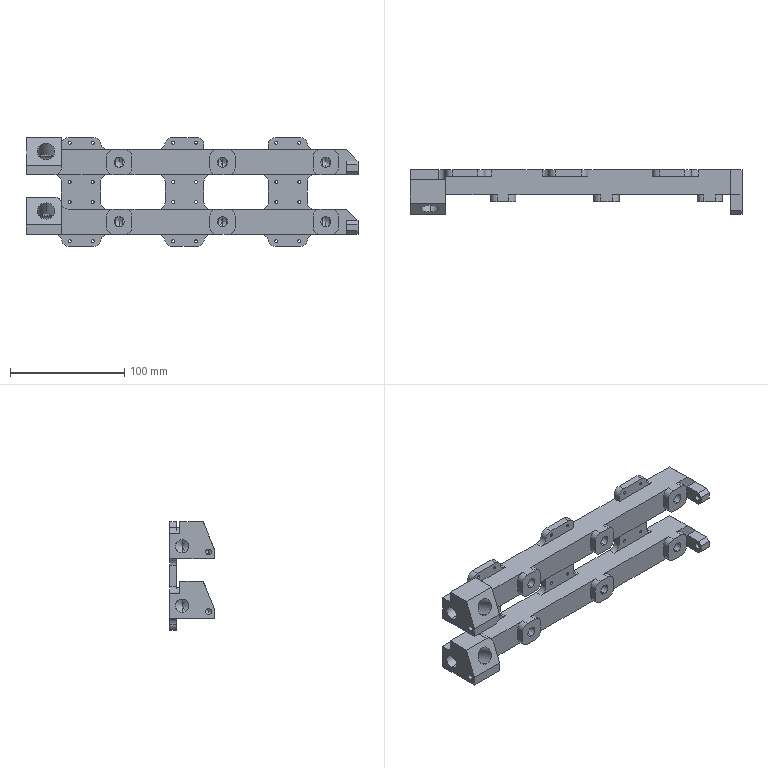CAM job | NX | 3+2 milling, drilling | part box 290 x 39.082 x 95 mm | stock box 300 x 49.082 x 95.918 mm
Tools:
number,name,description,diameter,corner_radius,flute_length,length,flutes
3,V4,定心钻D4,4.0,0.0,43.0,75.0,2
1,V10,定心钻D10,10.0,0.0,87.0,133.0,2
4,D4_J,D4,4.0,0.0,12.0,50.0,2
9,D6,D6,6.0,0.0,16.0,60.0,2
7,D8,D8,8.0,0.0,20.0,60.0,2
4,D8_J,D8,8.0,0.0,20.0,60.0,2
3,D10_J,D10,10.0,0.0,25.0,75.0,2
2,D12,D12,12.0,0.0,30.0,75.0,2
2,D16,D16,16.0,0.0,45.0,100.0,2
0,D4R0.5,圆鼻铣刀,4.0,0.5,12.0,50.0,2
1,D63R0.8,方肩铣刀片,40.0,0.8,15.0,80.0,2
2,DJ8-45,DJ8-32,8.0,0.0,4.0,60.0,2
13,Z2.5,Z2.5直柄钻头,2.5,0.0,30.0,57.0,2
16,Z5,Z5直柄钻头,5.0,0.0,52.0,86.0,2
2,Z6.8,Z6.8直柄钻头,6.8,0.0,69.0,109.0,2
14,M3X0.5,公制-铝用螺旋槽丝攻,2.5,0.0,11.0,18.0,2
17,M6X1,公制-铝用螺旋槽丝攻,5.0,0.0,19.0,30.0,2
3,M8X1.25,公制-铝用螺旋槽丝攻,6.5,0.0,22.0,25.0,2
0,M12X1.75,公制-铝用螺旋槽丝攻,10.3,0.0,29.0,32.0,2
3,D12-DRILL,Drilling Tool,12.0,0.0,35.0,50.0,2
18,G4-1,Thread Mill,9.9,0.0,20.0,50.0,2
11,G8-1,Thread Mill,7.7,0.0,30.0,50.0,2
5,D10.5,Drilling Tool,10.5,0.0,35.0,50.0,2
6,G3-8,Thread Mill,13.4,0.0,30.0,50.0,30
8,D2.5,Milling Tool-5 Parameters,2.5,0.0,50.0,75.0,2
10,D8.7,Drilling Tool,8.7,0.0,35.0,50.0,2
12,D30面刀,Milling Tool-5 Parameters,40.0,0.0,50.0,75.0,2
Operations:
program,operation,operation_type,tool,method,geometry_group,spindle_rpm,surface_speed,feed_per_tooth,feed_cut,feed_plunge,cut_length_mm,path_length_mm,cut_time_min,machine_time_min
ROUGHING-1,PLANAR_MILL_1,PlanarMilling,D63R0.8,METHOD,ROUGHING-1,3500.0,692.0,0.1429,1000.0,100.0,708.0,1327.087,0.708,0.7699
ROUGHING-1,DRILLING,Operation,DJ8-45,METHOD,ROUGHING-1,3000.0,0.0,0.0,200.0,0.0,9.0,249.415,0.045,0.069
ROUGHING-1,DRILLING_COPY,Operation,D12-DRILL,METHOD,ROUGHING-1,2000.0,0.0,0.0,200.0,0.0,96.0,423.415,0.48,0.5127
ROUGHING-2,ADAPTIVE-MILLING,CavityMilling,D16,METHOD,W1,5500.0,188.0,0.25,2500.0,100.0,60469.944,68342.892,24.188,24.975
ROUGHING-2,LINE-FINISHING,PlanarMilling,D16,METHOD,W1,3500.0,75.0,0.15,1000.0,100.0,952.628,1085.392,1.116,1.129
ROUGHING-2,ONE-CUT-FACE_1,VolumeBased25DMillingOperation,D16,METHOD,ROUGHING-1,3500.0,175.0,0.1429,1000.0,100.0,193.895,768.935,0.1939,0.2514
ROUGHING-2,LINE-CONTOUR,PlanarMilling,D10_J,METHOD,W1,5000.0,188.0,0.3,3000.0,100.0,3631.699,3891.799,1.364,1.39
M00,ADAPTIVE-MILLING_COPY,CavityMilling,D16,METHOD,W1,5500.0,188.0,0.25,2500.0,100.0,20777.618,22815.978,8.311,8.515
BRIDGE-PLATE,DRILLING_1,Operation,V10,METHOD,BRIDGE-PLATE,2000.0,62.0,0.05,200.0,0.0,18.0,525.505,0.09,0.1408
BRIDGE-PLATE,DRILLING_1_COPY,Operation,V10,METHOD,BRIDGE-PLATE,2000.0,62.0,0.05,200.0,0.0,42.0,820.986,0.21,0.2879
BRIDGE-PLATE,DRILLING_2,Operation,Z6.8,METHOD,BRIDGE-PLATE,2500.0,53.0,0.04,200.0,0.0,92.0,738.086,0.46,0.5246
BRIDGE-PLATE,DRILLING_2_COPY,Operation,M8X1.25,METHOD,BRIDGE-PLATE,300.0,6.0,0.0021,1.25,0.0,52.0,658.086,41.6,41.661
BRIDGE-PLATE,PLANAR_MILL_2,PlanarMilling,D4_J,METHOD,BRIDGE-PLATE,6500.0,81.0,0.0308,400.0,100.0,1225.499,1687.788,3.064,3.11
BRIDGE-PLATE,DRILLING_3,Operation,D10.5,METHOD,BRIDGE-PLATE,1500.0,49.0,0.05,150.0,0.0,46.0,245.05,0.3067,0.3266
BRIDGE-PLATE,PLANAR_MILL_3,PlanarMilling,V10,METHOD,BRIDGE-PLATE,3000.0,94.0,0.1,600.0,100.0,78.479,284.479,0.1308,0.1514
BRIDGE-PLATE,DRILLING_3_COPY,Operation,M12X1.75,METHOD,BRIDGE-PLATE,300.0,9.0,0.0029,1.75,0.0,26.0,205.05,14.857,14.875
4AXIS-1,ONE-CUT-FACE,VolumeBased25DMillingOperation,D12,METHOD,4AXIS-1,6000.0,226.0,0.1,1200.0,100.0,177.929,754.87,0.1483,0.206
4AXIS-1,LINE-FINISHING_COPY,PlanarMilling,D12,METHOD,4AXIS-1,6000.0,226.0,0.0833,1000.0,100.0,1883.053,2016.018,2.147,2.16
4AXIS-1,LINE-FINISHING_COPY_COPY_1,PlanarMilling,D12,METHOD,4AXIS-1,6000.0,226.0,0.0833,1000.0,100.0,614.738,1847.938,0.6147,0.7381
4AXIS-1,LINE-FINISHING_COPY_COPY_1_COPY,PlanarMilling,D12,METHOD,4AXIS-1,6000.0,226.0,0.0833,1000.0,100.0,112.468,300.804,0.1125,0.1313
4AXIS-1,ONE-CUT-FACE_COPY,VolumeBased25DMillingOperation,D12,METHOD,4AXIS-1,6000.0,226.0,0.0667,800.0,100.0,177.929,755.67,0.2224,0.2802
4AXIS-1,LINE-FINISHING_COPY_COPY_1_COPY_1,PlanarMilling,D12,METHOD,4AXIS-1,6000.0,226.0,0.0667,800.0,100.0,617.275,1852.495,0.7716,0.8951
4AXIS-1,LINE-FINISHING_COPY_COPY_1_COPY_COPY,PlanarMilling,D12,METHOD,4AXIS-1,6000.0,226.0,0.0833,800.0,100.0,113.775,302.987,0.1571,0.176
4AXIS-1,LINE-FINISHING_COPY_COPY,PlanarMilling,D12,METHOD,4AXIS-1,6000.0,226.0,0.0667,800.0,100.0,3764.045,3947.544,4.807,4.826
4AXIS-1,LINE-FINISHING_COPY_COPY_COPY_COPY,PlanarMilling,D12,METHOD,4AXIS-1,6000.0,226.0,0.0667,800.0,100.0,1189.536,2171.253,1.509,1.607
4AXIS-1,PLANAR_MILL_4,PlanarMilling,V4,METHOD,4AXIS-1,3000.0,37.0,0.1667,1000.0,100.0,287.491,1324.128,0.2875,0.3912
4AXIS-1,2D-SPOT-DRILL_3,Operation,D8_J,METHOD,4AXIS-1,2000.0,18.0,0.05,200.0,0.0,42.0,697.536,0.21,0.2756
4AXIS-1,SURFACE-CONTOUR_COPY,SurfaceContour,D4R0.5,METHOD,4AXIS-1,6000.0,150.0,0.25,3000.0,100.0,2279.565,2461.064,0.7599,0.778
4AXIS-2-SETUP,SURFACE-CONTOUR,SurfaceContour,D4R0.5,METHOD,4AXIS-1,6000.0,150.0,0.25,3000.0,100.0,11146.427,11216.56,3.716,3.723
4AXIS-2,ZIGZAG-FACE,VolumeBased25DMillingOperation,D12,METHOD,4AXIS-2,6000.0,1187.0,0.125,1500.0,100.0,389.962,525.191,0.26,0.2735
4AXIS-2,ONE-CUT-FACE_2,VolumeBased25DMillingOperation,D30面刀,METHOD,4AXIS-2,3000.0,376.0,0.1,600.0,100.0,85.0,100.041,0.1417,0.1432
4AXIS-2,ONE-CUT-FACE_2_COPY,VolumeBased25DMillingOperation,D30面刀,METHOD,4AXIS-2,3000.0,376.0,0.1,600.0,100.0,85.0,139.0,0.1417,0.1471
4AXIS-2,PLANAR_MILL_6,PlanarMilling,D8,METHOD,4AXIS-2,6500.0,100.0,0.1178,1200.0,100.0,1513.542,1557.583,1.261,1.266
4AXIS-2,PLANAR_MILL_6_COPY,PlanarMilling,D8,METHOD,4AXIS-2,6500.0,100.0,0.1178,1200.0,100.0,1513.542,1596.542,1.261,1.27
4AXIS-2,PLANAR_MILL_5,PlanarMilling,D8_J,METHOD,4AXIS-2,3000.0,100.0,0.1178,600.0,100.0,49.012,71.053,0.0817,0.0839
4AXIS-2,PLANAR_MILL_5_COPY,PlanarMilling,D8_J,METHOD,4AXIS-2,3000.0,100.0,0.1178,600.0,100.0,49.012,110.012,0.0817,0.0878
4AXIS-2,THREAD_MILLING,ThreadMilling,G3-8,METHOD,4AXIS-2,4500.0,189.0,0.0011,150.0,100.0,105.18,179.53,0.7012,0.7086
4AXIS-2,THREAD_MILLING_COPY,ThreadMilling,G3-8,METHOD,4AXIS-2,4500.0,189.0,0.0011,150.0,100.0,105.18,218.489,0.7012,0.7125
4AXIS-3,PLANAR_MILL_7,PlanarMilling,D2.5,METHOD,4AXIS-3,6500.0,51.0,0.1538,2000.0,100.0,2251.159,5957.939,1.126,1.496
4AXIS-3,PLANAR_MILL_7_COPY,PlanarMilling,D2.5,METHOD,4AXIS-3,6500.0,51.0,0.1538,2000.0,100.0,2800.0,7584.0,1.4,1.878
4AXIS-3,FLOOR_FACING_1,VolumeBased25DMillingOperation,D2.5,METHOD,4AXIS-3,6500.0,51.0,0.1538,500.0,100.0,519.872,898.712,1.04,1.078
4AXIS-3,PLANAR_MILL_7_COPY_1,PlanarMilling,D2.5,METHOD,4AXIS-3,6500.0,51.0,0.0462,500.0,100.0,258.561,654.771,0.5171,0.5567
4AXIS-3,PLANAR_MILL_7_COPY_COPY,PlanarMilling,D2.5,METHOD,4AXIS-3,6500.0,51.0,0.0462,500.0,100.0,321.6,813.282,0.6432,0.6924
4AXIS-4,FLOOR_FACING_COPY,VolumeBased25DMillingOperation,D12,METHOD,4AXIS-1,6500.0,245.0,0.0923,1200.0,100.0,748.676,1661.006,0.6239,0.7151
4AXIS-4,FLOOR_FACING,VolumeBased25DMillingOperation,D12,METHOD,4AXIS-1,6500.0,245.0,0.0923,1200.0,100.0,1523.194,2675.765,1.269,1.385
4AXIS-4,FLOOR_FACING_COPY_1,VolumeBased25DMillingOperation,D12,METHOD,4AXIS-1,6500.0,245.0,0.0923,1200.0,100.0,555.326,1096.162,0.4628,0.5169
4AXIS-4,LINE-FINISHING_1_COPY,PlanarMilling,D12,METHOD,4AXIS-1,6500.0,245.0,0.0923,1200.0,100.0,648.604,899.66,0.549,0.5741
4AXIS-4,LINE-FINISHING_COPY_COPY_2_COPY_COPY,PlanarMilling,D12,METHOD,4AXIS-1,6000.0,226.0,0.0667,800.0,100.0,271.766,631.918,0.4139,0.45
4AXIS-4,LINE-FINISHING_COPY_COPY_2_COPY_COPY_COPY,PlanarMilling,D12,METHOD,4AXIS-1,6000.0,226.0,0.0667,800.0,100.0,38.083,172.848,0.0534,0.0669
4AXIS-4,PLANAR_MILL,PlanarMilling,D12,METHOD,4AXIS-1,6000.0,226.0,0.0667,800.0,100.0,325.759,1145.303,0.4072,0.4892
4AXIS-4,PLANAR_MILL_COPY_1,PlanarMilling,D12,METHOD,4AXIS-1,6000.0,226.0,0.0667,800.0,100.0,349.779,1203.278,0.4372,0.5226
4AXIS-4,FLOOR_FACING_2,VolumeBased25DMillingOperation,D6,METHOD,4AXIS-1,6500.0,122.0,0.0923,1200.0,100.0,1916.939,4041.195,1.597,1.81
4AXIS-4,FLOOR_FACING_2_COPY,VolumeBased25DMillingOperation,D6,METHOD,4AXIS-1,6500.0,122.0,0.0462,600.0,100.0,159.745,390.976,0.2662,0.2894
4AXIS-4,PLANAR_MILL_COPY,PlanarMilling,D6,METHOD,4AXIS-1,1061.0,100.0,0.1178,250.0,100.0,170.85,624.507,0.6834,0.7288
4AXIS-4,PLANAR_MILL_COPY_COPY,PlanarMilling,D6,METHOD,4AXIS-1,1061.0,100.0,0.1178,250.0,100.0,194.23,638.889,0.7769,0.8214
4AXIS-4,PLANAR_MILL_9,PlanarMilling,D30面刀,METHOD,4AXIS-1,3500.0,329.0,0.1143,800.0,100.0,378.0,915.942,0.4725,0.5263
4AXIS-4,FLOOR_FACING_COPY_2,VolumeBased25DMillingOperation,D12,METHOD,4AXIS-1,6000.0,245.0,0.0923,800.0,100.0,1523.194,2676.965,1.904,2.019
4AXIS-4,FLOOR_FACING_COPY_1_COPY,VolumeBased25DMillingOperation,D12,METHOD,4AXIS-1,6000.0,245.0,0.0923,800.0,100.0,555.548,1096.985,0.6944,0.7486
4AXIS-4,LINE-FINISHING_1_COPY_COPY,PlanarMilling,D12,METHOD,4AXIS-1,6000.0,245.0,0.0923,800.0,100.0,1297.105,2313.467,1.647,1.749
4AXIS-4,LINE-FINISHING_COPY_COPY_2_COPY_COPY_COPY_1,PlanarMilling,D12,METHOD,4AXIS-1,6000.0,226.0,0.0667,800.0,100.0,540.165,900.317,0.6752,0.7112
4AXIS-4,LINE-FINISHING_COPY_COPY_2_COPY_COPY_COPY_COPY,PlanarMilling,D12,METHOD,4AXIS-1,6000.0,226.0,0.0667,800.0,100.0,76.566,316.558,0.0957,0.1197
4AXIS-4,PLANAR_MILL_COPY_2,PlanarMilling,D12,METHOD,4AXIS-1,6000.0,226.0,0.0667,800.0,100.0,324.345,1145.032,0.4054,0.4875
4AXIS-4,PLANAR_MILL_COPY_1_COPY,PlanarMilling,D12,METHOD,4AXIS-1,6000.0,226.0,0.0667,800.0,100.0,347.894,1202.638,0.4349,0.5203
4AXIS-4,2D-SPOT-DRILL_2,Operation,D8_J,METHOD,4AXIS-1,2000.0,18.0,0.05,200.0,0.0,24.0,530.927,0.12,0.1707
4AXIS-4,2D-SPOT-DRILL_3_COPY,Operation,D8_J,METHOD,4AXIS-1,2000.0,18.0,0.05,200.0,0.0,42.0,530.938,0.21,0.2589
4AXIS-4,2D-SPOT-DRILL_2_COPY,Operation,D8.7,METHOD,4AXIS-1,2000.0,54.0,0.05,200.0,0.0,120.0,722.927,0.6,0.6603
4AXIS-4,PLANAR_MILL_8,PlanarMilling,D8_J,METHOD,4AXIS-1,4500.0,113.0,0.0667,600.0,100.0,159.162,979.728,0.2653,0.3473
4AXIS-4,THREAD_MILLING_1,ThreadMilling,G8-1,METHOD,4AXIS-1,5500.0,133.0,0.0182,200.0,100.0,251.22,1393.618,1.256,1.37
4AXIS-4,PLANAR-CHAMFER_2_COPY,PlanarMilling,V4,METHOD,4AXIS-1,4000.0,50.0,0.125,1000.0,100.0,123.297,301.584,0.1233,0.1411
4AXIS-4,PLANAR-CHAMFER_2_COPY_COPY,PlanarMilling,V4,METHOD,4AXIS-1,4000.0,50.0,0.125,1000.0,100.0,68.0,368.6,0.068,0.0981
4AXIS-4,PLANAR-CHAMFER_2,PlanarMilling,V4,METHOD,4AXIS-1,4000.0,50.0,0.125,1000.0,100.0,585.823,1472.424,0.5858,0.6745
4AXIS-4,PLANAR-CHAMFER_2_COPY_1,PlanarMilling,V4,METHOD,4AXIS-1,4000.0,50.0,0.125,1000.0,100.0,427.25,1121.038,0.4272,0.4966
4AXIS-4,PLANAR-CHAMFER_2_COPY_1_COPY,PlanarMilling,V4,METHOD,4AXIS-1,4000.0,50.0,0.125,1000.0,100.0,434.716,1070.656,0.4347,0.4983
4AXIS-4,PLANAR-CHAMFER_2_COPY_1_COPY_COPY,PlanarMilling,V4,METHOD,4AXIS-1,4000.0,50.0,0.125,1000.0,100.0,208.016,1171.649,0.208,0.3044
四轴5,ZIGZAG-FACE_2,VolumeBased25DMillingOperation,D30面刀,METHOD,四轴5,3500.0,1187.0,0.1,1000.0,100.0,1401.986,1455.786,1.402,1.407
四轴5,ZIGZAG-FACE_2_COPY,VolumeBased25DMillingOperation,D30面刀,METHOD,四轴5,3500.0,1187.0,0.1,600.0,100.0,1401.986,1455.986,2.337,2.342
四轴5,2D-SPOT-DRILL,Operation,D8_J,METHOD,四轴5,2000.0,18.0,0.05,200.0,0.0,84.0,918.247,0.42,0.5034
四轴5,PLANAR-CHAMFER_COPY,PlanarMilling,D8_J,METHOD,四轴5,3500.0,113.0,0.0417,1000.0,100.0,323.747,526.947,0.3237,0.3441
四轴5,2D-SPOT-DRILL_COPY,Operation,Z2.5,METHOD,四轴5,2000.0,18.0,0.05,200.0,0.0,252.0,1254.247,1.26,1.36
四轴5,2D-SPOT-DRILL_COPY_COPY,Operation,M3X0.5,METHOD,四轴5,300.0,18.0,0.05,0.5,0.0,204.0,1158.247,408.0,408.095
四轴5,FLOOR-WALL-ZIGZAG,VolumeBased25DMillingOperation,D8,METHOD,四轴5,6000.0,188.0,0.25,1200.0,100.0,1382.682,2021.847,1.152,1.216
四轴5,LINE-CONTOUR_1_COPY,PlanarMilling,D8,METHOD,四轴5,6000.0,188.0,0.3,1200.0,100.0,304.56,575.068,0.2538,0.2809
四轴5,FLOOR-WALL-ZIGZAG_COPY,VolumeBased25DMillingOperation,D8,METHOD,四轴5,6000.0,188.0,0.25,600.0,100.0,230.447,430.247,0.3841,0.4041
四轴5,LINE-CONTOUR_1,PlanarMilling,D8,METHOD,四轴5,6000.0,188.0,0.3,600.0,100.0,128.762,318.248,0.2146,0.2336
四轴5,PLANAR-CHAMFER,PlanarMilling,D8_J,METHOD,四轴5,3500.0,113.0,0.0417,1000.0,100.0,942.801,999.801,0.9428,0.9485
四轴6,PLANAR_MILL_11_COPY,PlanarMilling,D30面刀,METHOD,四轴6,3000.0,376.0,0.1,600.0,100.0,178.165,389.679,0.2969,0.3181
四轴6,PLANAR_MILL_11,PlanarMilling,D30面刀,METHOD,四轴6,3000.0,376.0,0.1,600.0,100.0,178.165,389.879,0.2969,0.3181
四轴6,PLANAR_MILL_10,PlanarMilling,D8,METHOD,四轴6,6500.0,100.0,0.1178,600.0,100.0,79.882,601.254,0.1331,0.1853
四轴6,PLANAR-CHAMFER_1,PlanarMilling,D8_J,METHOD,四轴6,3500.0,113.0,0.0417,800.0,100.0,68.826,238.836,0.086,0.103
四轴6,2D-SPOT-DRILL_1,Operation,D8_J,METHOD,四轴6,2000.0,18.0,0.05,200.0,0.0,10.0,134.038,0.05,0.0624
四轴6,2D-SPOT-DRILL_1_COPY,Operation,Z5,METHOD,四轴6,2000.0,18.0,0.05,200.0,0.0,36.0,186.038,0.18,0.195
四轴6,2D-SPOT-DRILL_1_COPY_COPY,Operation,M6X1,METHOD,四轴6,300.0,18.0,0.05,1.0,0.0,32.0,178.038,32.0,32.015
四轴6,THREAD-MILLING,ThreadMilling,G4-1,METHOD,四轴6,4500.0,51.0,0.0714,200.0,100.0,960.699,1306.453,4.803,4.838
4AXIS-7,2D-SPOT-DRILL_1_COPY_1,Operation,D8_J,METHOD,4AXIS-7,2000.0,18.0,0.05,200.0,0.0,10.0,134.038,0.05,0.0624
4AXIS-7,2D-SPOT-DRILL_1_COPY_COPY_1,Operation,Z5,METHOD,4AXIS-7,2000.0,18.0,0.05,200.0,0.0,36.0,186.038,0.18,0.195
4AXIS-7,2D-SPOT-DRILL_1_COPY_COPY_COPY,Operation,M6X1,METHOD,4AXIS-7,300.0,18.0,0.05,1.0,0.0,32.0,178.038,32.0,32.015
PROGRAM,PLANAR_MILL_12,PlanarMilling,D8,METHOD,MCS,4500.0,113.0,0.1111,1000.0,100.0,280.0,906.8,0.28,0.3427
PROGRAM,PLANAR_MILL_12_COPY,PlanarMilling,D8,METHOD,MCS,4500.0,113.0,0.0889,800.0,100.0,56.0,172.2,0.07,0.0816